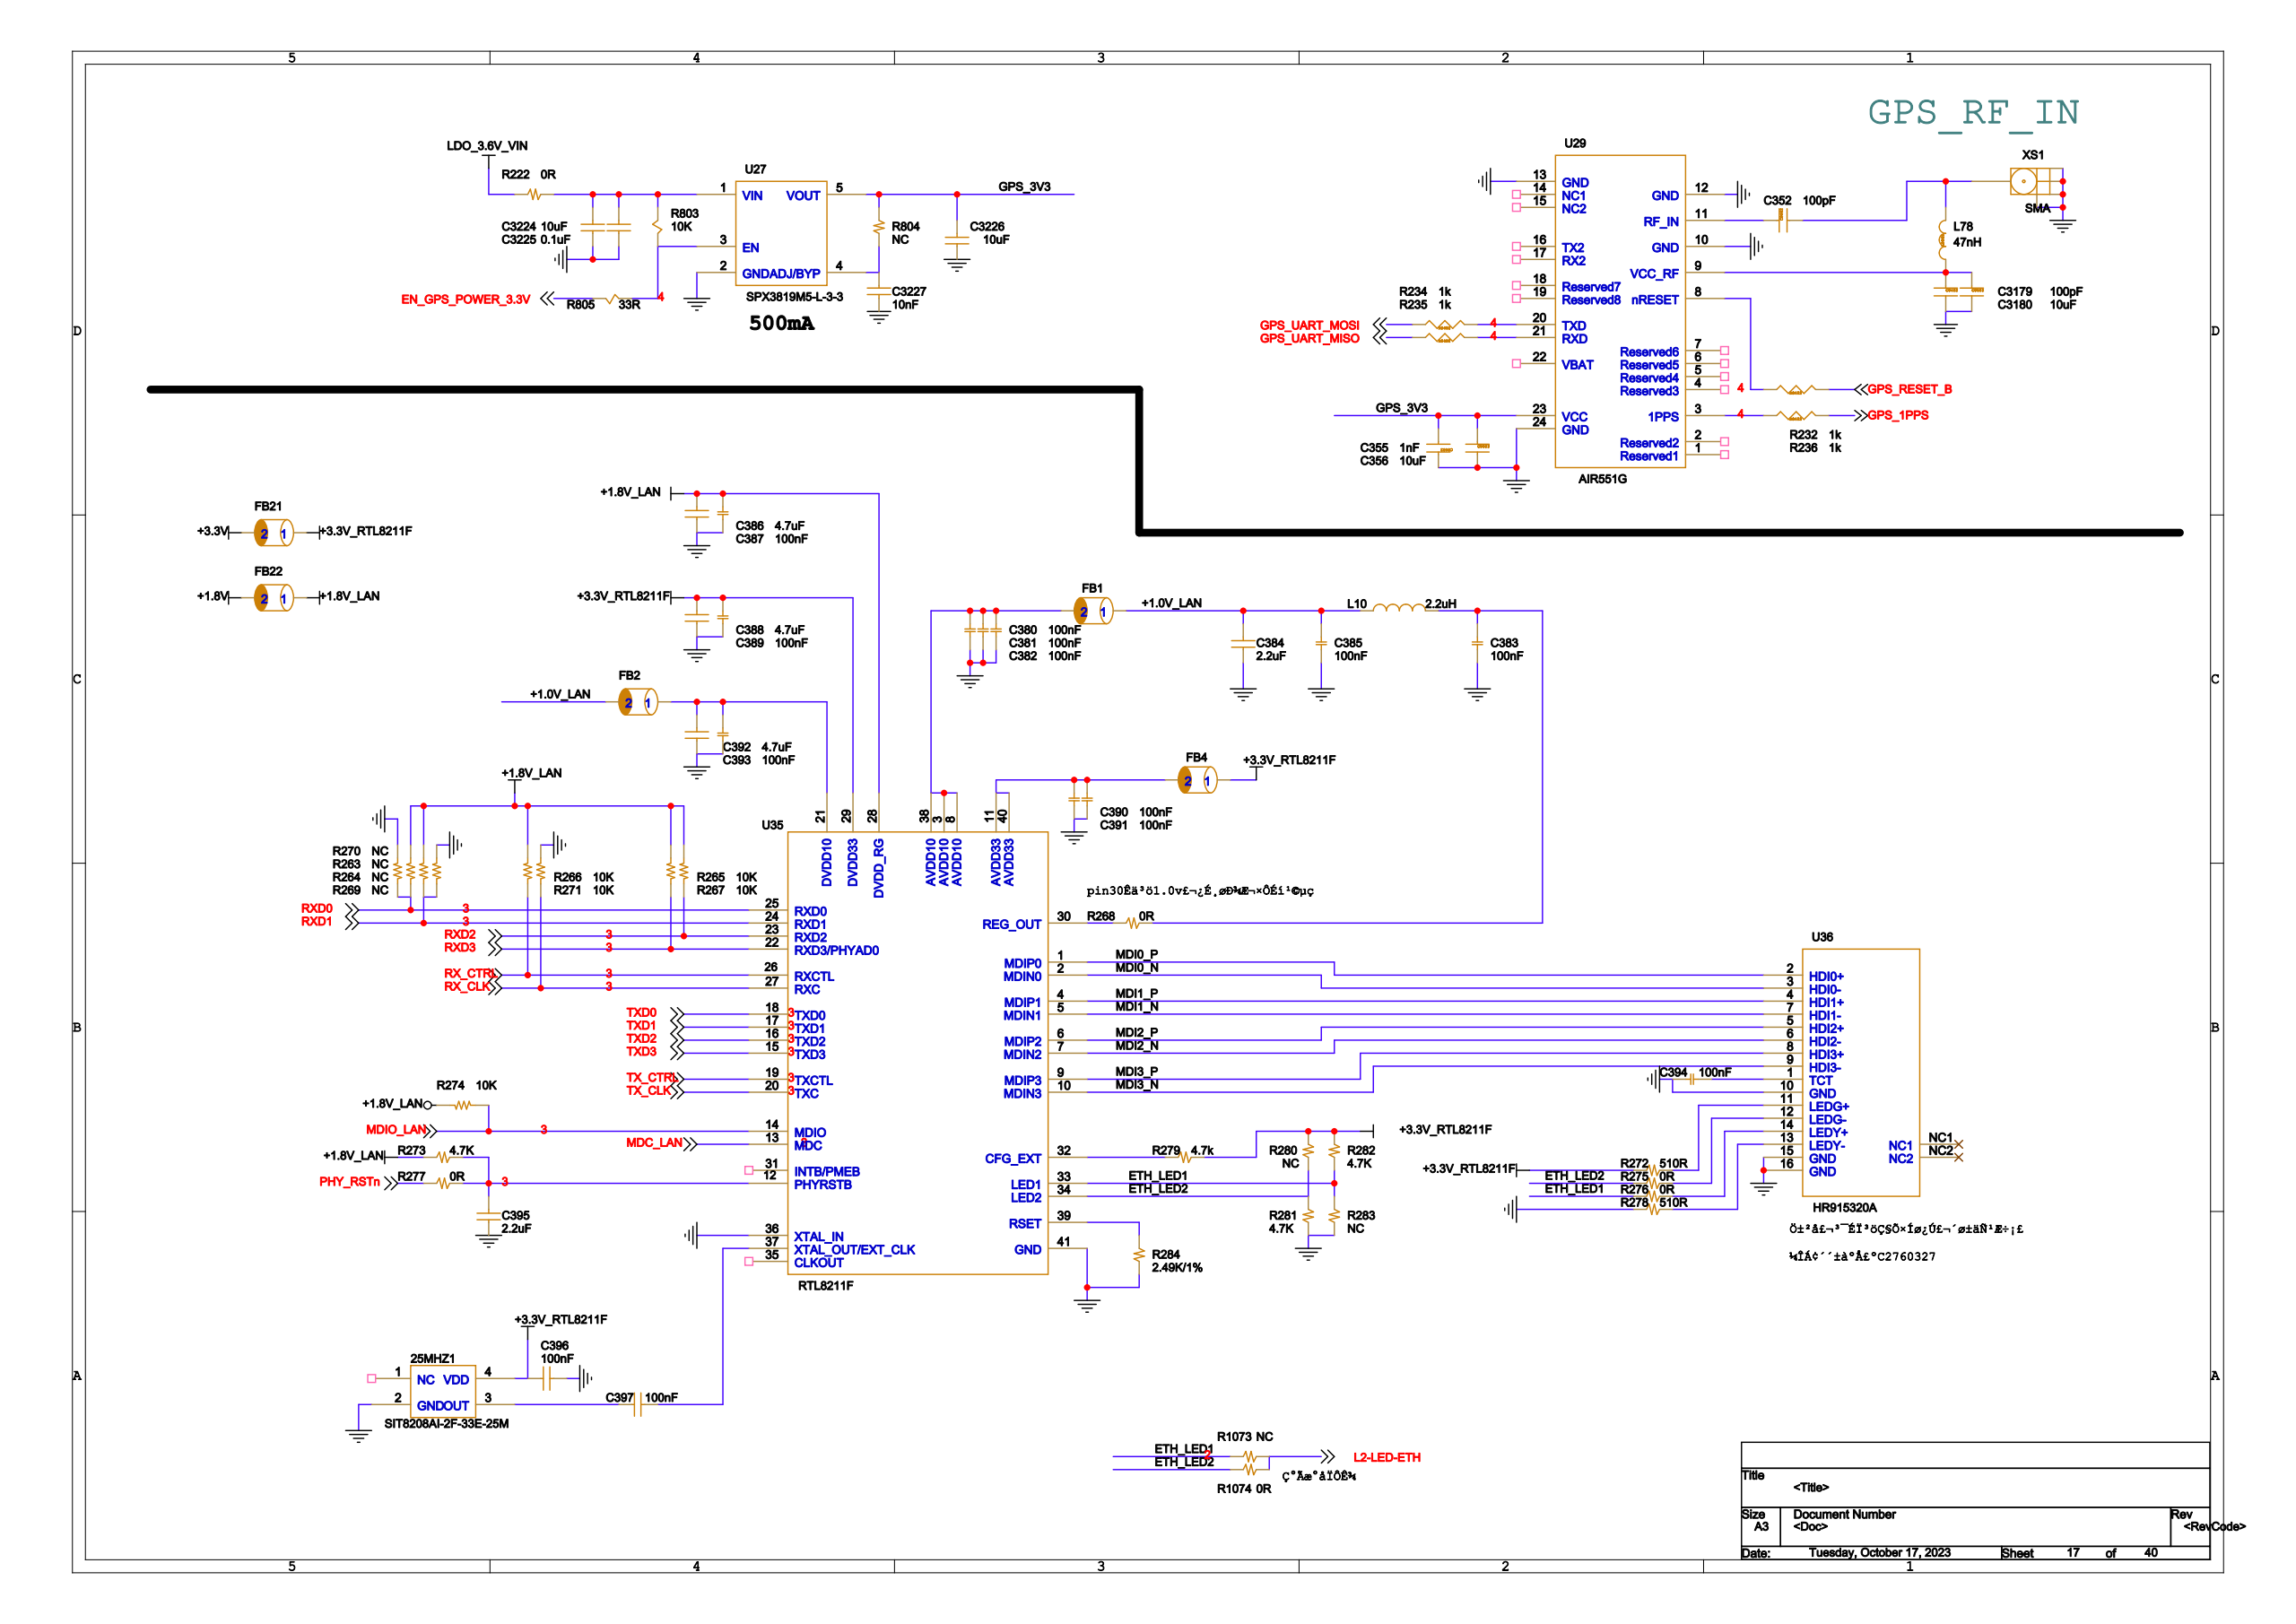Circuit board | Cadence Allegro | 1793 parts | 1223 nets | one sheet of the schematic
Parts on this sheet (reference | value | footprint):
25MHZ1 | SIT8208AI-2F-33E-25M | 3225
C352 | 100pF | C0402
C355 | 1nF | C0402
C356 | 10uF | C0402
C380 | 100nF | C0402
C381 | 100nF | C0402
C382 | 100nF | C0402
C383 | 100nF | C0402
C384 | 2.2uF | C0402
C385 | 100nF | C0402
C386 | 4.7uF | C0402
C387 | 100nF | C0402
C388 | 4.7uF | C0402
C389 | 100nF | C0402
C390 | 100nF | C0402
C391 | 100nF | C0402
C392 | 4.7uF | C0402
C393 | 100nF | C0402
C394 | 100nF | C0402
C395 | 2.2uF | C0402
C396 | 100nF | C0402
C397 | 100nF | C0402
C3179 | 100pF | C0402
C3180 | 10uF | C0402
C3224 | 10uF | C0402
C3225 | 0.1uF | C0402
C3226 | 10uF | C0402
C3227 | 10nF | C0402
FB1 | BLM18PG121SN1 | FB0603
FB2 | BLM18PG121SN1 | FB0603
FB4 | BLM18PG121SN1 | FB0603
FB21 | BLM18PG121SN1 | FB0603
FB22 | BLM18PG121SN1 | FB0603
L10 | 2.2uH | I0603
L78 | 47nH | L0603
R222 | 0R | R0402
R232 | 1k | R0402
R234 | 1k | R0402
R235 | 1k | R0402
R236 | 1k | R0402
R263 | NC | R0402
R264 | NC | R0402
R265 | 10K | R0402
R266 | 10K | R0402
R267 | 10K | R0402
R268 | 0R | R0402
R269 | NC | R0402
R270 | NC | R0402
R271 | 10K | R0402
R272 | 510R | R0402
R273 | 4.7K | R0402
R274 | 10K | R0402
R275 | 0R | R0402
R276 | 0R | R0402
R277 | 0R | R0402
R278 | 510R | R0402
R279 | 4.7K | R0402
R280 | NC | R0402
R281 | 4.7K | R0402
R282 | 4.7K | R0402
R283 | NC | R0402
R284 | 2.49K/1% | R0402
R803 | 10K | R0402
R804 | NC | R0402
R805 | 33R | R0402
R1073 | NC | R0402
R1074 | 0R | R0402
U27 | SPX3819M5-L-3-3 | SOT-23-5
U29 | AIR551G | AIR551G
U35 | RTL8211F | QFN40_500X500
U36 | HR915320A | RJ45-TH_HR915320A
XS1 | SMA | SMA_5X5MM
Nets of these parts (net: part-pin ...):
GND: 25MHZ1-2 C355-1 C356-2 C380-2 C381-2 C382-2 C383-2 C384-1 C385-2 C386-1 C387-2 C388-1 C389-2 C390-2 C391-2 C392-1 C393-2 C394-1 C395-1 C396-2 C3179-2 C3180-2 C3224-1 C3225-1 C3226-1 C3227-2 R269-2 R270-2 R271-1 R278-2 R281-2 R283-2 R284-2 U27-2 U29-10 U29-12 U29-13 U29-24 U36-10 U36-15 U36-16 XS1-2 XS1-3 XS1-4 XS1-5 U35-36 U35-41
+3.3V: FB21-2
LDO_3.6V_VIN: R222-1
MDI0_P: U36-2 U35-1
MDI0_N: U36-3 U35-2
MDI1_P: U36-4 U35-4
MDI1_N: U36-7 U35-5
MDI2_P: U36-5 U35-6
MDI2_N: U36-6 U35-7
MDI3_P: U36-8 U35-9
MDI3_N: U36-9 U35-10
N1365247: R272-1 U36-11
N1365427: R275-1 U36-12
N1365423: R276-1 U36-14
N1365407: R278-1 U36-13
N1365387: C394-2 U36-1
N18701353: C3179-1 C3180-1 L78-1 U29-9
GPS_3V3: C355-2 C356-1 C3226-2 R804-1 U27-5 U29-23
+1.8V: FB22-2
N18701751: C3224-2 C3225-2 R222-2 R803-2 U27-1
+1.0V_LAN: C384-2 C385-1 FB1-1 FB2-2 L10-1
N1365523: C395-2 R273-1 R277-2 U35-12
L2-LED-ETH: R1073-2 R1074-2
N1365363: 25MHZ1-3 C397-1
+3.3V_RTL8211F: 25MHZ1-4 C388-2 C389-1 C396-1 FB4-1 FB21-1 R272-2 R279-1 R280-2 R282-2 U35-29
N1364849: C380-1 C381-1 C382-1 FB1-2 U35-3 U35-8 U35-38
N1366081: C390-1 C391-1 FB4-2 U35-11 U35-40
N1365683: R279-2 U35-32
N16691786: C392-2 C393-1 FB2-1 U35-21
+1.8V_LAN: C386-2 C387-1 FB22-1 R263-2 R264-2 R265-2 R266-2 R267-2 R273-2 R274-2 U35-28
ETH_LED1: R276-2 R282-1 R283-1 R1073-1 U35-33
ETH_LED2: R275-2 R280-1 R281-1 R1074-1 U35-34
MDC_LAN: U35-13
MDIO_LAN: R274-1 U35-14
N1364801: R268-2 U35-30
N1365783: R284-1 U35-39
RX_CLK: R271-2 U35-27
RX_CTRL: R266-1 U35-26
RXD0: R263-1 R270-1 U35-25
RXD1: R264-1 R269-1 U35-24
RXD2: R267-1 U35-23
RXD3: R265-1 U35-22
TX_CLK: U35-20
TX_CTRL: U35-19
TXD0: U35-18
TXD1: U35-17
TXD2: U35-16
TXD3: U35-15
N1365367: C397-2 U35-37
N18701309: C352-2 L78-2 XS1-1
N18701826: C3227-1 R804-2 U27-4
N18701335: C352-1 U29-11
N1364813: C383-1 L10-2 R268-1
N18701822: R803-1 R805-1 U27-3
EN_GPS_POWER_3.3V: R805-2
PHY_RSTN: R277-1
N18701373: R232-1 U29-8
GPS_RESET_B: R232-2
GPS_UART_MOSI: R234-1
N18701409: R234-2 U29-20
GPS_UART_MISO: R235-1
N18701415: R235-2 U29-21
N18701458: R236-1 U29-3
GPS_1PPS: R236-2